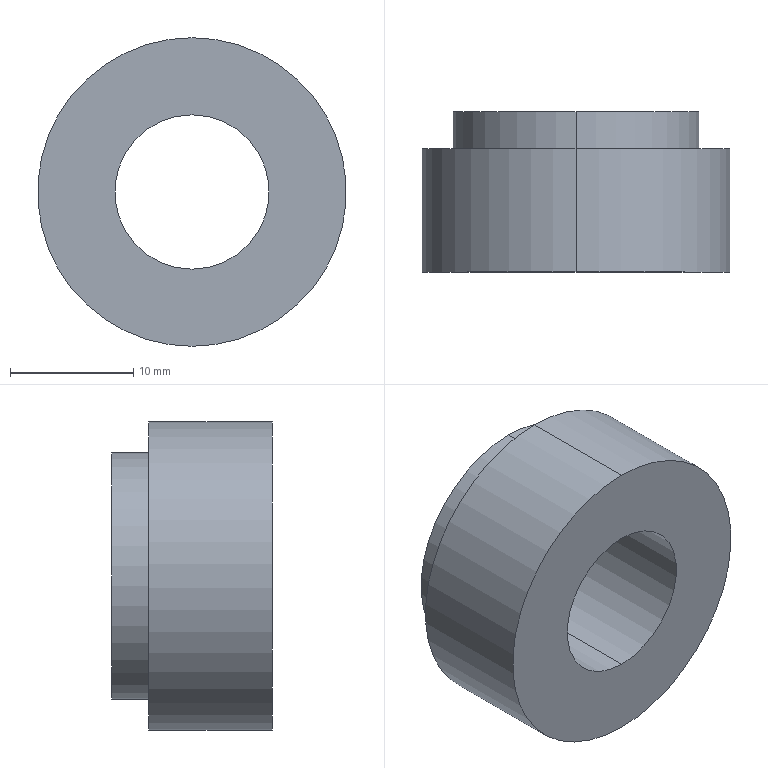Part | SolidWorks | features HoleWzd 1, Revolution 1 | 1 solid | 9 faces | box 25 x 13 x 25 mm | volume 4256 mm3 | cylinder 6 | plane 3 | commonest cylinder face diameters 12.5 x2 20 x2 25 x2
STEP:
#1=CARTESIAN_POINT('',(0.,13.,-6.25));
#2=VERTEX_POINT('',#1);
#3=CARTESIAN_POINT('',(0.,13.,6.25));
#4=VERTEX_POINT('',#3);
#5=CARTESIAN_POINT('',(0.,13.,0.));
#6=DIRECTION('',(0.,1.,0.));
#7=DIRECTION('',(0.,0.,1.));
#8=AXIS2_PLACEMENT_3D('',#5,#6,#7);
#9=CIRCLE('',#8,6.25);
#10=EDGE_CURVE('',#2,#4,#9,.T.);
#11=ORIENTED_EDGE('',*,*,#10,.T.);
#12=CARTESIAN_POINT('',(0.,0.,6.25));
#13=VERTEX_POINT('',#12);
#14=CARTESIAN_POINT('',(0.,0.,6.25));
#15=DIRECTION('',(0.,-1.,0.));
#16=VECTOR('',#15,1000.);
#17=LINE('',#14,#16);
#18=EDGE_CURVE('',#4,#13,#17,.T.);
#19=ORIENTED_EDGE('',*,*,#18,.T.);
#20=CARTESIAN_POINT('',(0.,0.,-6.25));
#21=VERTEX_POINT('',#20);
#22=CARTESIAN_POINT('',(0.,0.,0.));
#23=DIRECTION('',(0.,-1.,0.));
#24=DIRECTION('',(0.,0.,-1.));
#25=AXIS2_PLACEMENT_3D('',#22,#23,#24);
#26=CIRCLE('',#25,6.25);
#27=EDGE_CURVE('',#13,#21,#26,.T.);
#28=ORIENTED_EDGE('',*,*,#27,.T.);
#29=CARTESIAN_POINT('',(0.,0.,-6.25));
#30=DIRECTION('',(0.,-1.,0.));
#31=VECTOR('',#30,1000.);
#32=LINE('',#29,#31);
#33=EDGE_CURVE('',#2,#21,#32,.T.);
#34=ORIENTED_EDGE('',*,*,#33,.F.);
#35=EDGE_LOOP('',(#11,#19,#28,#34));
#36=FACE_OUTER_BOUND('',#35,.T.);
#37=CARTESIAN_POINT('',(0.,0.,0.));
#38=DIRECTION('',(0.,-1.,0.));
#39=DIRECTION('',(0.,0.,-1.));
#40=AXIS2_PLACEMENT_3D('',#37,#38,#39);
#41=CYLINDRICAL_SURFACE('',#40,6.25);
#42=ADVANCED_FACE('',(#36),#41,.F.);
#43=CARTESIAN_POINT('',(0.,13.,-10.));
#44=VERTEX_POINT('',#43);
#45=CARTESIAN_POINT('',(0.,13.,10.));
#46=VERTEX_POINT('',#45);
#47=CARTESIAN_POINT('',(0.,13.,0.));
#48=DIRECTION('',(0.,-1.,0.));
#49=DIRECTION('',(0.,0.,-1.));
#50=AXIS2_PLACEMENT_3D('',#47,#48,#49);
#51=CIRCLE('',#50,10.);
#52=EDGE_CURVE('',#44,#46,#51,.T.);
#53=ORIENTED_EDGE('',*,*,#52,.T.);
#54=CARTESIAN_POINT('',(0.,10.,10.));
#55=VERTEX_POINT('',#54);
#56=CARTESIAN_POINT('',(0.,0.,10.));
#57=DIRECTION('',(0.,-1.,0.));
#58=VECTOR('',#57,1000.);
#59=LINE('',#56,#58);
#60=EDGE_CURVE('',#46,#55,#59,.T.);
#61=ORIENTED_EDGE('',*,*,#60,.T.);
#62=CARTESIAN_POINT('',(0.,10.,-10.));
#63=VERTEX_POINT('',#62);
#64=CARTESIAN_POINT('',(0.,10.,0.));
#65=DIRECTION('',(0.,-1.,0.));
#66=DIRECTION('',(0.,0.,-1.));
#67=AXIS2_PLACEMENT_3D('',#64,#65,#66);
#68=CIRCLE('',#67,10.);
#69=EDGE_CURVE('',#63,#55,#68,.T.);
#70=ORIENTED_EDGE('',*,*,#69,.F.);
#71=CARTESIAN_POINT('',(0.,0.,-10.));
#72=DIRECTION('',(0.,-1.,0.));
#73=VECTOR('',#72,1000.);
#74=LINE('',#71,#73);
#75=EDGE_CURVE('',#44,#63,#74,.T.);
#76=ORIENTED_EDGE('',*,*,#75,.F.);
#77=EDGE_LOOP('',(#53,#61,#70,#76));
#78=FACE_OUTER_BOUND('',#77,.T.);
#79=CARTESIAN_POINT('',(0.,0.,0.));
#80=DIRECTION('',(0.,-1.,0.));
#81=DIRECTION('',(0.,0.,-1.));
#82=AXIS2_PLACEMENT_3D('',#79,#80,#81);
#83=CYLINDRICAL_SURFACE('',#82,10.);
#84=ADVANCED_FACE('',(#78),#83,.T.);
#85=CARTESIAN_POINT('',(0.,10.,-12.5));
#86=VERTEX_POINT('',#85);
#87=CARTESIAN_POINT('',(0.,10.,12.5));
#88=VERTEX_POINT('',#87);
#89=CARTESIAN_POINT('',(0.,10.,0.));
#90=DIRECTION('',(0.,-1.,0.));
#91=DIRECTION('',(0.,0.,-1.));
#92=AXIS2_PLACEMENT_3D('',#89,#90,#91);
#93=CIRCLE('',#92,12.5);
#94=EDGE_CURVE('',#86,#88,#93,.T.);
#95=ORIENTED_EDGE('',*,*,#94,.T.);
#96=CARTESIAN_POINT('',(0.,0.,12.5));
#97=VERTEX_POINT('',#96);
#98=CARTESIAN_POINT('',(0.,0.,12.5));
#99=DIRECTION('',(0.,-1.,0.));
#100=VECTOR('',#99,1000.);
#101=LINE('',#98,#100);
#102=EDGE_CURVE('',#88,#97,#101,.T.);
#103=ORIENTED_EDGE('',*,*,#102,.T.);
#104=CARTESIAN_POINT('',(0.,0.,-12.5));
#105=VERTEX_POINT('',#104);
#106=CARTESIAN_POINT('',(0.,0.,0.));
#107=DIRECTION('',(0.,-1.,0.));
#108=DIRECTION('',(0.,0.,-1.));
#109=AXIS2_PLACEMENT_3D('',#106,#107,#108);
#110=CIRCLE('',#109,12.5);
#111=EDGE_CURVE('',#105,#97,#110,.T.);
#112=ORIENTED_EDGE('',*,*,#111,.F.);
#113=CARTESIAN_POINT('',(0.,0.,-12.5));
#114=DIRECTION('',(0.,-1.,0.));
#115=VECTOR('',#114,1000.);
#116=LINE('',#113,#115);
#117=EDGE_CURVE('',#86,#105,#116,.T.);
#118=ORIENTED_EDGE('',*,*,#117,.F.);
#119=EDGE_LOOP('',(#95,#103,#112,#118));
#120=FACE_OUTER_BOUND('',#119,.T.);
#121=CARTESIAN_POINT('',(0.,0.,0.));
#122=DIRECTION('',(0.,-1.,0.));
#123=DIRECTION('',(0.,0.,-1.));
#124=AXIS2_PLACEMENT_3D('',#121,#122,#123);
#125=CYLINDRICAL_SURFACE('',#124,12.5);
#126=ADVANCED_FACE('',(#120),#125,.T.);
#127=CARTESIAN_POINT('',(0.,0.,0.));
#128=DIRECTION('',(0.,-1.,0.));
#129=DIRECTION('',(0.,0.,-1.));
#130=AXIS2_PLACEMENT_3D('',#127,#128,#129);
#131=CIRCLE('',#130,6.25);
#132=EDGE_CURVE('',#21,#13,#131,.T.);
#133=ORIENTED_EDGE('',*,*,#132,.F.);
#134=ORIENTED_EDGE('',*,*,#27,.F.);
#135=EDGE_LOOP('',(#133,#134));
#136=FACE_BOUND('',#135,.T.);
#137=ORIENTED_EDGE('',*,*,#111,.T.);
#138=CARTESIAN_POINT('',(0.,0.,0.));
#139=DIRECTION('',(0.,-1.,0.));
#140=DIRECTION('',(0.,0.,-1.));
#141=AXIS2_PLACEMENT_3D('',#138,#139,#140);
#142=CIRCLE('',#141,12.5);
#143=EDGE_CURVE('',#97,#105,#142,.T.);
#144=ORIENTED_EDGE('',*,*,#143,.T.);
#145=EDGE_LOOP('',(#137,#144));
#146=FACE_OUTER_BOUND('',#145,.T.);
#147=CARTESIAN_POINT('',(0.,0.,0.));
#148=DIRECTION('',(0.,-1.,0.));
#149=DIRECTION('',(0.,0.,-1.));
#150=AXIS2_PLACEMENT_3D('',#147,#148,#149);
#151=PLANE('',#150);
#152=ADVANCED_FACE('',(#136,#146),#151,.T.);
#153=ORIENTED_EDGE('',*,*,#102,.F.);
#154=CARTESIAN_POINT('',(0.,10.,0.));
#155=DIRECTION('',(0.,-1.,0.));
#156=DIRECTION('',(0.,0.,-1.));
#157=AXIS2_PLACEMENT_3D('',#154,#155,#156);
#158=CIRCLE('',#157,12.5);
#159=EDGE_CURVE('',#88,#86,#158,.T.);
#160=ORIENTED_EDGE('',*,*,#159,.T.);
#161=ORIENTED_EDGE('',*,*,#117,.T.);
#162=ORIENTED_EDGE('',*,*,#143,.F.);
#163=EDGE_LOOP('',(#153,#160,#161,#162));
#164=FACE_OUTER_BOUND('',#163,.T.);
#165=CARTESIAN_POINT('',(0.,0.,0.));
#166=DIRECTION('',(0.,-1.,0.));
#167=DIRECTION('',(0.,0.,-1.));
#168=AXIS2_PLACEMENT_3D('',#165,#166,#167);
#169=CYLINDRICAL_SURFACE('',#168,12.5);
#170=ADVANCED_FACE('',(#164),#169,.T.);
#171=ORIENTED_EDGE('',*,*,#69,.T.);
#172=CARTESIAN_POINT('',(0.,10.,0.));
#173=DIRECTION('',(0.,-1.,0.));
#174=DIRECTION('',(0.,0.,-1.));
#175=AXIS2_PLACEMENT_3D('',#172,#173,#174);
#176=CIRCLE('',#175,10.);
#177=EDGE_CURVE('',#55,#63,#176,.T.);
#178=ORIENTED_EDGE('',*,*,#177,.T.);
#179=EDGE_LOOP('',(#171,#178));
#180=FACE_BOUND('',#179,.T.);
#181=ORIENTED_EDGE('',*,*,#94,.F.);
#182=ORIENTED_EDGE('',*,*,#159,.F.);
#183=EDGE_LOOP('',(#181,#182));
#184=FACE_OUTER_BOUND('',#183,.T.);
#185=CARTESIAN_POINT('',(12.5,10.,0.));
#186=DIRECTION('',(0.,1.,0.));
#187=DIRECTION('',(0.,0.,1.));
#188=AXIS2_PLACEMENT_3D('',#185,#186,#187);
#189=PLANE('',#188);
#190=ADVANCED_FACE('',(#180,#184),#189,.T.);
#191=ORIENTED_EDGE('',*,*,#60,.F.);
#192=CARTESIAN_POINT('',(0.,13.,0.));
#193=DIRECTION('',(0.,-1.,0.));
#194=DIRECTION('',(0.,0.,-1.));
#195=AXIS2_PLACEMENT_3D('',#192,#193,#194);
#196=CIRCLE('',#195,10.);
#197=EDGE_CURVE('',#46,#44,#196,.T.);
#198=ORIENTED_EDGE('',*,*,#197,.T.);
#199=ORIENTED_EDGE('',*,*,#75,.T.);
#200=ORIENTED_EDGE('',*,*,#177,.F.);
#201=EDGE_LOOP('',(#191,#198,#199,#200));
#202=FACE_OUTER_BOUND('',#201,.T.);
#203=CARTESIAN_POINT('',(0.,0.,0.));
#204=DIRECTION('',(0.,-1.,0.));
#205=DIRECTION('',(0.,0.,-1.));
#206=AXIS2_PLACEMENT_3D('',#203,#204,#205);
#207=CYLINDRICAL_SURFACE('',#206,10.);
#208=ADVANCED_FACE('',(#202),#207,.T.);
#209=ORIENTED_EDGE('',*,*,#10,.F.);
#210=CARTESIAN_POINT('',(0.,13.,0.));
#211=DIRECTION('',(0.,1.,0.));
#212=DIRECTION('',(0.,0.,1.));
#213=AXIS2_PLACEMENT_3D('',#210,#211,#212);
#214=CIRCLE('',#213,6.25);
#215=EDGE_CURVE('',#4,#2,#214,.T.);
#216=ORIENTED_EDGE('',*,*,#215,.F.);
#217=EDGE_LOOP('',(#209,#216));
#218=FACE_BOUND('',#217,.T.);
#219=ORIENTED_EDGE('',*,*,#52,.F.);
#220=ORIENTED_EDGE('',*,*,#197,.F.);
#221=EDGE_LOOP('',(#219,#220));
#222=FACE_OUTER_BOUND('',#221,.T.);
#223=CARTESIAN_POINT('',(10.,13.,0.));
#224=DIRECTION('',(0.,1.,0.));
#225=DIRECTION('',(0.,0.,1.));
#226=AXIS2_PLACEMENT_3D('',#223,#224,#225);
#227=PLANE('',#226);
#228=ADVANCED_FACE('',(#218,#222),#227,.T.);
#229=ORIENTED_EDGE('',*,*,#18,.F.);
#230=ORIENTED_EDGE('',*,*,#215,.T.);
#231=ORIENTED_EDGE('',*,*,#33,.T.);
#232=ORIENTED_EDGE('',*,*,#132,.T.);
#233=EDGE_LOOP('',(#229,#230,#231,#232));
#234=FACE_OUTER_BOUND('',#233,.T.);
#235=CARTESIAN_POINT('',(0.,0.,0.));
#236=DIRECTION('',(0.,-1.,0.));
#237=DIRECTION('',(0.,0.,-1.));
#238=AXIS2_PLACEMENT_3D('',#235,#236,#237);
#239=CYLINDRICAL_SURFACE('',#238,6.25);
#240=ADVANCED_FACE('',(#234),#239,.F.);
#241=CLOSED_SHELL('',(#42,#84,#126,#152,#170,#190,#208,#228,#240));
#242=MANIFOLD_SOLID_BREP('',#241);
#243=CARTESIAN_POINT('',(0.,0.,0.));
#244=DIRECTION('',(0.,0.,1.));
#245=DIRECTION('',(1.,0.,0.));
#246=AXIS2_PLACEMENT_3D('',#243,#244,#245);
#247=(LENGTH_UNIT()NAMED_UNIT(*)SI_UNIT(.MILLI.,.METRE.));
#248=UNCERTAINTY_MEASURE_WITH_UNIT(LENGTH_MEASURE(0.00001),#247,'','');
#249=(NAMED_UNIT(*)PLANE_ANGLE_UNIT()SI_UNIT($,.RADIAN.));
#250=(NAMED_UNIT(*)SI_UNIT($,.STERADIAN.)SOLID_ANGLE_UNIT());
#251=(GEOMETRIC_REPRESENTATION_CONTEXT(3)GLOBAL_UNCERTAINTY_ASSIGNED_CONTEXT((#248))GLOBAL_UNIT_ASSIGNED_CONTEXT((#247,#249,#250))REPRESENTATION_CONTEXT('',''));
#252=ADVANCED_BREP_SHAPE_REPRESENTATION('',(#242,#246),#251);